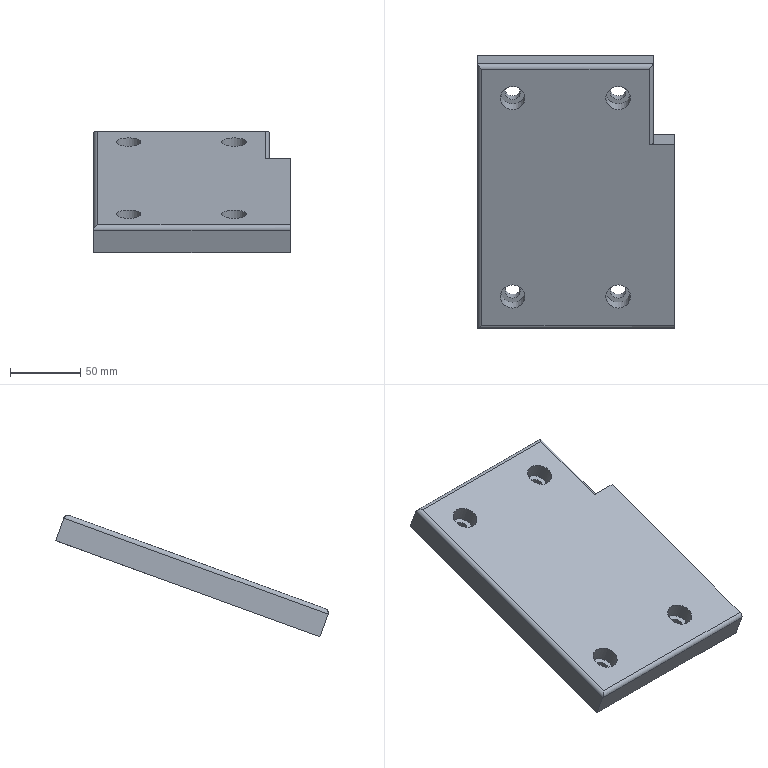Part | NX | features solid 2 | 1 solid | 24 faces | box 140 x 193.934 x 86.353 mm | volume 526407 mm3 | plane 12 | cylinder 12 | commonest cylinder face diameters 6 x4 11 x4 17.5 x4
STEP:
#1=CARTESIAN_POINT('',(540.,942.377,-265.264));
#2=VERTEX_POINT('',#1);
#3=CARTESIAN_POINT('',(540.,998.758,-244.742));
#4=VERTEX_POINT('',#3);
#5=CARTESIAN_POINT('',(540.,810.726,-313.181));
#6=DIRECTION('',(0.,0.9397,0.342));
#7=VECTOR('',#6,1000.);
#8=LINE('',#5,#7);
#9=EDGE_CURVE('',#2,#4,#8,.T.);
#10=ORIENTED_EDGE('',*,*,#9,.F.);
#11=CARTESIAN_POINT('',(540.,948.191,-281.238));
#12=VERTEX_POINT('',#11);
#13=CARTESIAN_POINT('',(540.,941.316,-262.351));
#14=DIRECTION('',(0.,0.342,-0.9397));
#15=VECTOR('',#14,1000.);
#16=LINE('',#13,#15);
#17=EDGE_CURVE('',#2,#12,#16,.T.);
#18=ORIENTED_EDGE('',*,*,#17,.T.);
#19=CARTESIAN_POINT('',(540.,1004.573,-260.717));
#20=VERTEX_POINT('',#19);
#21=CARTESIAN_POINT('',(540.,816.446,-329.19));
#22=DIRECTION('',(0.,0.9397,0.342));
#23=VECTOR('',#22,1000.);
#24=LINE('',#21,#23);
#25=EDGE_CURVE('',#12,#20,#24,.T.);
#26=ORIENTED_EDGE('',*,*,#25,.T.);
#27=CARTESIAN_POINT('',(540.,997.698,-241.829));
#28=DIRECTION('',(0.,0.342,-0.9397));
#29=VECTOR('',#28,1000.);
#30=LINE('',#27,#29);
#31=EDGE_CURVE('',#4,#20,#30,.T.);
#32=ORIENTED_EDGE('',*,*,#31,.F.);
#33=EDGE_LOOP('',(#10,#18,#26,#32));
#34=FACE_BOUND('',#33,.T.);
#35=CARTESIAN_POINT('',(540.,809.665,-310.268));
#36=DIRECTION('',(1.,0.,0.));
#37=DIRECTION('',(0.,0.9397,0.342));
#38=AXIS2_PLACEMENT_3D('',#35,#36,#37);
#39=PLANE('',#38);
#40=ADVANCED_FACE('',(#34),#39,.T.);
#41=CARTESIAN_POINT('',(415.,810.82,-313.146));
#42=VERTEX_POINT('',#41);
#43=CARTESIAN_POINT('',(555.,810.82,-313.146));
#44=VERTEX_POINT('',#43);
#45=CARTESIAN_POINT('',(543.95,810.82,-313.146));
#46=DIRECTION('',(-1.,0.,0.));
#47=VECTOR('',#46,1000.);
#48=LINE('',#45,#47);
#49=EDGE_CURVE('',#42,#44,#48,.F.);
#50=ORIENTED_EDGE('',*,*,#49,.T.);
#51=CARTESIAN_POINT('',(555.,812.613,-309.301));
#52=VERTEX_POINT('',#51);
#53=CARTESIAN_POINT('',(555.,813.639,-312.12));
#54=DIRECTION('',(1.,0.,0.));
#55=DIRECTION('',(0.,1.,0.));
#56=AXIS2_PLACEMENT_3D('',#53,#54,#55);
#57=CIRCLE('',#56,3.);
#58=EDGE_CURVE('',#44,#52,#57,.F.);
#59=ORIENTED_EDGE('',*,*,#58,.T.);
#60=CARTESIAN_POINT('',(418.,812.613,-309.301));
#61=VERTEX_POINT('',#60);
#62=CARTESIAN_POINT('',(427.4,812.613,-309.301));
#63=DIRECTION('',(-1.,0.,0.));
#64=VECTOR('',#63,1000.);
#65=LINE('',#62,#64);
#66=EDGE_CURVE('',#52,#61,#65,.T.);
#67=ORIENTED_EDGE('',*,*,#66,.T.);
#68=CARTESIAN_POINT('',(418.,813.639,-312.12));
#69=DIRECTION('',(0.7071,-0.6645,-0.2418));
#70=DIRECTION('',(-0.7071,-0.6645,-0.2418));
#71=AXIS2_PLACEMENT_3D('',#68,#69,#70);
#72=ELLIPSE('',#71,4.243,3.);
#73=EDGE_CURVE('',#61,#42,#72,.T.);
#74=ORIENTED_EDGE('',*,*,#73,.T.);
#75=EDGE_LOOP('',(#50,#59,#67,#74));
#76=FACE_BOUND('',#75,.T.);
#77=CARTESIAN_POINT('',(427.4,813.639,-312.12));
#78=DIRECTION('',(-1.,0.,0.));
#79=DIRECTION('',(0.,1.,0.));
#80=AXIS2_PLACEMENT_3D('',#77,#78,#79);
#81=CYLINDRICAL_SURFACE('',#80,3.);
#82=ADVANCED_FACE('',(#76),#81,.T.);
#83=CARTESIAN_POINT('',(537.,994.913,-242.949));
#84=VERTEX_POINT('',#83);
#85=CARTESIAN_POINT('',(537.,941.351,-262.444));
#86=VERTEX_POINT('',#85);
#87=CARTESIAN_POINT('',(537.,809.606,-310.396));
#88=DIRECTION('',(0.,0.9397,0.342));
#89=VECTOR('',#88,1000.);
#90=LINE('',#87,#89);
#91=EDGE_CURVE('',#84,#86,#90,.F.);
#92=ORIENTED_EDGE('',*,*,#91,.T.);
#93=CARTESIAN_POINT('',(537.,942.377,-265.264));
#94=DIRECTION('',(0.,-0.9397,-0.342));
#95=DIRECTION('',(-0.0602,0.3414,-0.938));
#96=AXIS2_PLACEMENT_3D('',#93,#94,#95);
#97=CIRCLE('',#96,3.);
#98=EDGE_CURVE('',#86,#2,#97,.F.);
#99=ORIENTED_EDGE('',*,*,#98,.T.);
#100=ORIENTED_EDGE('',*,*,#9,.T.);
#101=CARTESIAN_POINT('',(537.,995.939,-245.768));
#102=DIRECTION('',(0.7071,-0.6645,-0.2418));
#103=DIRECTION('',(0.7071,0.6645,0.2418));
#104=AXIS2_PLACEMENT_3D('',#101,#102,#103);
#105=ELLIPSE('',#104,4.243,3.);
#106=EDGE_CURVE('',#4,#84,#105,.T.);
#107=ORIENTED_EDGE('',*,*,#106,.T.);
#108=EDGE_LOOP('',(#92,#99,#100,#107));
#109=FACE_BOUND('',#108,.T.);
#110=CARTESIAN_POINT('',(537.,810.726,-313.181));
#111=DIRECTION('',(0.,0.9397,0.342));
#112=DIRECTION('',(0.,-0.342,0.9397));
#113=AXIS2_PLACEMENT_3D('',#110,#111,#112);
#114=CYLINDRICAL_SURFACE('',#113,3.);
#115=ADVANCED_FACE('',(#109),#114,.T.);
#116=CARTESIAN_POINT('',(555.,941.351,-262.444));
#117=VERTEX_POINT('',#116);
#118=CARTESIAN_POINT('',(540.,941.351,-262.444));
#119=DIRECTION('',(-1.,0.,0.));
#120=VECTOR('',#119,1000.);
#121=LINE('',#118,#120);
#122=EDGE_CURVE('',#86,#117,#121,.F.);
#123=ORIENTED_EDGE('',*,*,#122,.F.);
#124=ORIENTED_EDGE('',*,*,#91,.F.);
#125=CARTESIAN_POINT('',(418.,994.913,-242.949));
#126=VERTEX_POINT('',#125);
#127=CARTESIAN_POINT('',(427.4,994.913,-242.949));
#128=DIRECTION('',(-1.,0.,0.));
#129=VECTOR('',#128,1000.);
#130=LINE('',#127,#129);
#131=EDGE_CURVE('',#126,#84,#130,.F.);
#132=ORIENTED_EDGE('',*,*,#131,.F.);
#133=CARTESIAN_POINT('',(418.,809.606,-310.396));
#134=DIRECTION('',(0.,0.9397,0.342));
#135=VECTOR('',#134,1000.);
#136=LINE('',#133,#135);
#137=EDGE_CURVE('',#61,#126,#136,.T.);
#138=ORIENTED_EDGE('',*,*,#137,.F.);
#139=ORIENTED_EDGE('',*,*,#66,.F.);
#140=CARTESIAN_POINT('',(555.,809.7,-310.362));
#141=DIRECTION('',(0.,-0.9397,-0.342));
#142=VECTOR('',#141,1000.);
#143=LINE('',#140,#142);
#144=EDGE_CURVE('',#52,#117,#143,.F.);
#145=ORIENTED_EDGE('',*,*,#144,.T.);
#146=EDGE_LOOP('',(#123,#124,#132,#138,#139,#145));
#147=FACE_BOUND('',#146,.T.);
#148=CARTESIAN_POINT('',(440.,841.508,-298.784));
#149=VERTEX_POINT('',#148);
#150=CARTESIAN_POINT('',(440.,833.286,-301.777));
#151=DIRECTION('',(0.,-0.342,0.9397));
#152=DIRECTION('',(0.,0.9397,0.342));
#153=AXIS2_PLACEMENT_3D('',#150,#151,#152);
#154=CIRCLE('',#153,8.75);
#155=EDGE_CURVE('',#149,#149,#154,.T.);
#156=ORIENTED_EDGE('',*,*,#155,.F.);
#157=EDGE_LOOP('',(#156));
#158=FACE_BOUND('',#157,.T.);
#159=CARTESIAN_POINT('',(515.,841.508,-298.784));
#160=VERTEX_POINT('',#159);
#161=CARTESIAN_POINT('',(515.,833.286,-301.777));
#162=DIRECTION('',(0.,-0.342,0.9397));
#163=DIRECTION('',(0.,0.9397,0.342));
#164=AXIS2_PLACEMENT_3D('',#161,#162,#163);
#165=CIRCLE('',#164,8.75);
#166=EDGE_CURVE('',#160,#160,#165,.T.);
#167=ORIENTED_EDGE('',*,*,#166,.F.);
#168=EDGE_LOOP('',(#167));
#169=FACE_BOUND('',#168,.T.);
#170=CARTESIAN_POINT('',(515.,966.018,-253.466));
#171=VERTEX_POINT('',#170);
#172=CARTESIAN_POINT('',(515.,974.24,-250.474));
#173=DIRECTION('',(0.,0.342,-0.9397));
#174=DIRECTION('',(0.,-0.9397,-0.342));
#175=AXIS2_PLACEMENT_3D('',#172,#173,#174);
#176=CIRCLE('',#175,8.75);
#177=EDGE_CURVE('',#171,#171,#176,.F.);
#178=ORIENTED_EDGE('',*,*,#177,.F.);
#179=EDGE_LOOP('',(#178));
#180=FACE_BOUND('',#179,.T.);
#181=CARTESIAN_POINT('',(440.,966.018,-253.466));
#182=VERTEX_POINT('',#181);
#183=CARTESIAN_POINT('',(440.,974.24,-250.474));
#184=DIRECTION('',(0.,0.342,-0.9397));
#185=DIRECTION('',(0.,-0.9397,-0.342));
#186=AXIS2_PLACEMENT_3D('',#183,#184,#185);
#187=CIRCLE('',#186,8.75);
#188=EDGE_CURVE('',#182,#182,#187,.F.);
#189=ORIENTED_EDGE('',*,*,#188,.F.);
#190=EDGE_LOOP('',(#189));
#191=FACE_BOUND('',#190,.T.);
#192=CARTESIAN_POINT('',(427.4,809.606,-310.396));
#193=DIRECTION('',(0.,-0.342,0.9397));
#194=DIRECTION('',(0.,0.9397,0.342));
#195=AXIS2_PLACEMENT_3D('',#192,#193,#194);
#196=PLANE('',#195);
#197=ADVANCED_FACE('',(#147,#158,#169,#180,#191),#196,.T.);
#198=CARTESIAN_POINT('',(555.,816.634,-329.121));
#199=VERTEX_POINT('',#198);
#200=CARTESIAN_POINT('',(555.,809.759,-310.233));
#201=DIRECTION('',(0.,-0.342,0.9397));
#202=VECTOR('',#201,1000.);
#203=LINE('',#200,#202);
#204=EDGE_CURVE('',#199,#44,#203,.T.);
#205=ORIENTED_EDGE('',*,*,#204,.T.);
#206=ORIENTED_EDGE('',*,*,#49,.F.);
#207=CARTESIAN_POINT('',(415.,816.634,-329.121));
#208=VERTEX_POINT('',#207);
#209=CARTESIAN_POINT('',(415.,817.01,-330.155));
#210=DIRECTION('',(0.,-0.342,0.9397));
#211=VECTOR('',#210,1000.);
#212=LINE('',#209,#211);
#213=EDGE_CURVE('',#208,#42,#212,.T.);
#214=ORIENTED_EDGE('',*,*,#213,.F.);
#215=CARTESIAN_POINT('',(427.5,816.634,-329.121));
#216=DIRECTION('',(1.,0.,0.));
#217=VECTOR('',#216,1000.);
#218=LINE('',#215,#217);
#219=EDGE_CURVE('',#208,#199,#218,.T.);
#220=ORIENTED_EDGE('',*,*,#219,.T.);
#221=EDGE_LOOP('',(#205,#206,#214,#220));
#222=FACE_BOUND('',#221,.T.);
#223=CARTESIAN_POINT('',(543.95,817.01,-330.155));
#224=DIRECTION('',(0.,-0.9397,-0.342));
#225=DIRECTION('',(-1.,0.,0.));
#226=AXIS2_PLACEMENT_3D('',#223,#224,#225);
#227=PLANE('',#226);
#228=ADVANCED_FACE('',(#222),#227,.T.);
#229=ORIENTED_EDGE('',*,*,#25,.F.);
#230=CARTESIAN_POINT('',(555.,948.191,-281.238));
#231=VERTEX_POINT('',#230);
#232=CARTESIAN_POINT('',(540.,948.191,-281.238));
#233=DIRECTION('',(1.,0.,0.));
#234=VECTOR('',#233,1000.);
#235=LINE('',#232,#234);
#236=EDGE_CURVE('',#12,#231,#235,.T.);
#237=ORIENTED_EDGE('',*,*,#236,.T.);
#238=CARTESIAN_POINT('',(555.,816.446,-329.19));
#239=DIRECTION('',(0.,0.9397,0.342));
#240=VECTOR('',#239,1000.);
#241=LINE('',#238,#240);
#242=EDGE_CURVE('',#199,#231,#241,.T.);
#243=ORIENTED_EDGE('',*,*,#242,.F.);
#244=ORIENTED_EDGE('',*,*,#219,.F.);
#245=CARTESIAN_POINT('',(415.,1004.573,-260.717));
#246=VERTEX_POINT('',#245);
#247=CARTESIAN_POINT('',(415.,816.446,-329.19));
#248=DIRECTION('',(0.,-0.9397,-0.342));
#249=VECTOR('',#248,1000.);
#250=LINE('',#247,#249);
#251=EDGE_CURVE('',#246,#208,#250,.T.);
#252=ORIENTED_EDGE('',*,*,#251,.F.);
#253=CARTESIAN_POINT('',(526.6,1004.573,-260.717));
#254=DIRECTION('',(1.,0.,0.));
#255=VECTOR('',#254,1000.);
#256=LINE('',#253,#255);
#257=EDGE_CURVE('',#246,#20,#256,.T.);
#258=ORIENTED_EDGE('',*,*,#257,.T.);
#259=EDGE_LOOP('',(#229,#237,#243,#244,#252,#258));
#260=FACE_BOUND('',#259,.T.);
#261=CARTESIAN_POINT('',(440.,845.295,-318.69));
#262=VERTEX_POINT('',#261);
#263=CARTESIAN_POINT('',(440.,840.126,-320.571));
#264=DIRECTION('',(0.,-0.342,0.9397));
#265=DIRECTION('',(0.,0.9397,0.342));
#266=AXIS2_PLACEMENT_3D('',#263,#264,#265);
#267=CIRCLE('',#266,5.5);
#268=EDGE_CURVE('',#262,#262,#267,.T.);
#269=ORIENTED_EDGE('',*,*,#268,.T.);
#270=EDGE_LOOP('',(#269));
#271=FACE_BOUND('',#270,.T.);
#272=CARTESIAN_POINT('',(515.,845.295,-318.69));
#273=VERTEX_POINT('',#272);
#274=CARTESIAN_POINT('',(515.,840.126,-320.571));
#275=DIRECTION('',(0.,-0.342,0.9397));
#276=DIRECTION('',(0.,0.9397,0.342));
#277=AXIS2_PLACEMENT_3D('',#274,#275,#276);
#278=CIRCLE('',#277,5.5);
#279=EDGE_CURVE('',#273,#273,#278,.T.);
#280=ORIENTED_EDGE('',*,*,#279,.T.);
#281=EDGE_LOOP('',(#280));
#282=FACE_BOUND('',#281,.T.);
#283=CARTESIAN_POINT('',(515.,986.249,-267.387));
#284=VERTEX_POINT('',#283);
#285=CARTESIAN_POINT('',(515.,981.08,-269.268));
#286=DIRECTION('',(0.,-0.342,0.9397));
#287=DIRECTION('',(0.,0.9397,0.342));
#288=AXIS2_PLACEMENT_3D('',#285,#286,#287);
#289=CIRCLE('',#288,5.5);
#290=EDGE_CURVE('',#284,#284,#289,.T.);
#291=ORIENTED_EDGE('',*,*,#290,.T.);
#292=EDGE_LOOP('',(#291));
#293=FACE_BOUND('',#292,.T.);
#294=CARTESIAN_POINT('',(440.,986.249,-267.387));
#295=VERTEX_POINT('',#294);
#296=CARTESIAN_POINT('',(440.,981.08,-269.268));
#297=DIRECTION('',(0.,-0.342,0.9397));
#298=DIRECTION('',(0.,0.9397,0.342));
#299=AXIS2_PLACEMENT_3D('',#296,#297,#298);
#300=CIRCLE('',#299,5.5);
#301=EDGE_CURVE('',#295,#295,#300,.T.);
#302=ORIENTED_EDGE('',*,*,#301,.T.);
#303=EDGE_LOOP('',(#302));
#304=FACE_BOUND('',#303,.T.);
#305=CARTESIAN_POINT('',(544.05,816.446,-329.19));
#306=DIRECTION('',(0.,0.342,-0.9397));
#307=DIRECTION('',(0.,0.9397,0.342));
#308=AXIS2_PLACEMENT_3D('',#305,#306,#307);
#309=PLANE('',#308);
#310=ADVANCED_FACE('',(#260,#271,#282,#293,#304),#309,.T.);
#311=ORIENTED_EDGE('',*,*,#31,.T.);
#312=ORIENTED_EDGE('',*,*,#257,.F.);
#313=CARTESIAN_POINT('',(415.,998.758,-244.742));
#314=VERTEX_POINT('',#313);
#315=CARTESIAN_POINT('',(415.,997.698,-241.829));
#316=DIRECTION('',(0.,0.342,-0.9397));
#317=VECTOR('',#316,1000.);
#318=LINE('',#315,#317);
#319=EDGE_CURVE('',#314,#246,#318,.T.);
#320=ORIENTED_EDGE('',*,*,#319,.F.);
#321=CARTESIAN_POINT('',(526.6,998.758,-244.742));
#322=DIRECTION('',(-1.,0.,0.));
#323=VECTOR('',#322,1000.);
#324=LINE('',#321,#323);
#325=EDGE_CURVE('',#4,#314,#324,.T.);
#326=ORIENTED_EDGE('',*,*,#325,.F.);
#327=EDGE_LOOP('',(#311,#312,#320,#326));
#328=FACE_BOUND('',#327,.T.);
#329=CARTESIAN_POINT('',(526.6,997.698,-241.829));
#330=DIRECTION('',(0.,0.9397,0.342));
#331=DIRECTION('',(-1.,0.,0.));
#332=AXIS2_PLACEMENT_3D('',#329,#330,#331);
#333=PLANE('',#332);
#334=ADVANCED_FACE('',(#328),#333,.T.);
#335=ORIENTED_EDGE('',*,*,#319,.T.);
#336=ORIENTED_EDGE('',*,*,#251,.T.);
#337=ORIENTED_EDGE('',*,*,#213,.T.);
#338=CARTESIAN_POINT('',(415.,803.772,-315.712));
#339=DIRECTION('',(0.,0.9397,0.342));
#340=VECTOR('',#339,1000.);
#341=LINE('',#338,#340);
#342=EDGE_CURVE('',#314,#42,#341,.F.);
#343=ORIENTED_EDGE('',*,*,#342,.F.);
#344=EDGE_LOOP('',(#335,#336,#337,#343));
#345=FACE_BOUND('',#344,.T.);
#346=CARTESIAN_POINT('',(415.,809.928,-332.626));
#347=DIRECTION('',(-1.,0.,0.));
#348=DIRECTION('',(0.,0.9397,0.342));
#349=AXIS2_PLACEMENT_3D('',#346,#347,#348);
#350=PLANE('',#349);
#351=ADVANCED_FACE('',(#345),#350,.T.);
#352=ORIENTED_EDGE('',*,*,#268,.F.);
#353=EDGE_LOOP('',(#352));
#354=FACE_BOUND('',#353,.T.);
#355=CARTESIAN_POINT('',(440.,842.558,-311.172));
#356=VERTEX_POINT('',#355);
#357=CARTESIAN_POINT('',(440.,837.39,-313.053));
#358=DIRECTION('',(0.,-0.342,0.9397));
#359=DIRECTION('',(0.,0.9397,0.342));
#360=AXIS2_PLACEMENT_3D('',#357,#358,#359);
#361=CIRCLE('',#360,5.5);
#362=EDGE_CURVE('',#356,#356,#361,.T.);
#363=ORIENTED_EDGE('',*,*,#362,.T.);
#364=EDGE_LOOP('',(#363));
#365=FACE_BOUND('',#364,.T.);
#366=CARTESIAN_POINT('',(440.,850.387,-348.761));
#367=DIRECTION('',(0.,0.342,-0.9397));
#368=DIRECTION('',(0.,0.9397,0.342));
#369=AXIS2_PLACEMENT_3D('',#366,#367,#368);
#370=CYLINDRICAL_SURFACE('',#369,5.5);
#371=ADVANCED_FACE('',(#354,#365),#370,.F.);
#372=ORIENTED_EDGE('',*,*,#362,.F.);
#373=EDGE_LOOP('',(#372));
#374=FACE_BOUND('',#373,.T.);
#375=CARTESIAN_POINT('',(440.,845.612,-310.06));
#376=VERTEX_POINT('',#375);
#377=CARTESIAN_POINT('',(440.,837.39,-313.053));
#378=DIRECTION('',(0.,-0.342,0.9397));
#379=DIRECTION('',(0.,0.9397,0.342));
#380=AXIS2_PLACEMENT_3D('',#377,#378,#379);
#381=CIRCLE('',#380,8.75);
#382=EDGE_CURVE('',#376,#376,#381,.T.);
#383=ORIENTED_EDGE('',*,*,#382,.T.);
#384=EDGE_LOOP('',(#383));
#385=FACE_BOUND('',#384,.T.);
#386=CARTESIAN_POINT('',(452.,837.39,-313.053));
#387=DIRECTION('',(0.,0.342,-0.9397));
#388=DIRECTION('',(0.,0.9397,0.342));
#389=AXIS2_PLACEMENT_3D('',#386,#387,#388);
#390=PLANE('',#389);
#391=ADVANCED_FACE('',(#374,#385),#390,.F.);
#392=ORIENTED_EDGE('',*,*,#382,.F.);
#393=EDGE_LOOP('',(#392));
#394=FACE_BOUND('',#393,.T.);
#395=ORIENTED_EDGE('',*,*,#155,.T.);
#396=EDGE_LOOP('',(#395));
#397=FACE_BOUND('',#396,.T.);
#398=CARTESIAN_POINT('',(440.,833.286,-301.777));
#399=DIRECTION('',(0.,0.342,-0.9397));
#400=DIRECTION('',(0.,0.9397,0.342));
#401=AXIS2_PLACEMENT_3D('',#398,#399,#400);
#402=CYLINDRICAL_SURFACE('',#401,8.75);
#403=ADVANCED_FACE('',(#394,#397),#402,.F.);
#404=ORIENTED_EDGE('',*,*,#279,.F.);
#405=EDGE_LOOP('',(#404));
#406=FACE_BOUND('',#405,.T.);
#407=CARTESIAN_POINT('',(515.,842.558,-311.172));
#408=VERTEX_POINT('',#407);
#409=CARTESIAN_POINT('',(515.,837.39,-313.053));
#410=DIRECTION('',(0.,-0.342,0.9397));
#411=DIRECTION('',(0.,0.9397,0.342));
#412=AXIS2_PLACEMENT_3D('',#409,#410,#411);
#413=CIRCLE('',#412,5.5);
#414=EDGE_CURVE('',#408,#408,#413,.T.);
#415=ORIENTED_EDGE('',*,*,#414,.T.);
#416=EDGE_LOOP('',(#415));
#417=FACE_BOUND('',#416,.T.);
#418=CARTESIAN_POINT('',(515.,850.387,-348.761));
#419=DIRECTION('',(0.,0.342,-0.9397));
#420=DIRECTION('',(0.,0.9397,0.342));
#421=AXIS2_PLACEMENT_3D('',#418,#419,#420);
#422=CYLINDRICAL_SURFACE('',#421,5.5);
#423=ADVANCED_FACE('',(#406,#417),#422,.F.);
#424=ORIENTED_EDGE('',*,*,#414,.F.);
#425=EDGE_LOOP('',(#424));
#426=FACE_BOUND('',#425,.T.);
#427=CARTESIAN_POINT('',(515.,845.612,-310.06));
#428=VERTEX_POINT('',#427);
#429=CARTESIAN_POINT('',(515.,837.39,-313.053));
#430=DIRECTION('',(0.,-0.342,0.9397));
#431=DIRECTION('',(0.,0.9397,0.342));
#432=AXIS2_PLACEMENT_3D('',#429,#430,#431);
#433=CIRCLE('',#432,8.75);
#434=EDGE_CURVE('',#428,#428,#433,.T.);
#435=ORIENTED_EDGE('',*,*,#434,.T.);
#436=EDGE_LOOP('',(#435));
#437=FACE_BOUND('',#436,.T.);
#438=CARTESIAN_POINT('',(502.,837.39,-313.053));
#439=DIRECTION('',(0.,0.342,-0.9397));
#440=DIRECTION('',(0.,0.9397,0.342));
#441=AXIS2_PLACEMENT_3D('',#438,#439,#440);
#442=PLANE('',#441);
#443=ADVANCED_FACE('',(#426,#437),#442,.F.);
#444=ORIENTED_EDGE('',*,*,#434,.F.);
#445=EDGE_LOOP('',(#444));
#446=FACE_BOUND('',#445,.T.);
#447=ORIENTED_EDGE('',*,*,#166,.T.);
#448=EDGE_LOOP('',(#447));
#449=FACE_BOUND('',#448,.T.);
#450=CARTESIAN_POINT('',(515.,833.286,-301.777));
#451=DIRECTION('',(0.,0.342,-0.9397));
#452=DIRECTION('',(0.,0.9397,0.342));
#453=AXIS2_PLACEMENT_3D('',#450,#451,#452);
#454=CYLINDRICAL_SURFACE('',#453,8.75);
#455=ADVANCED_FACE('',(#446,#449),#454,.F.);
#456=ORIENTED_EDGE('',*,*,#290,.F.);
#457=EDGE_LOOP('',(#456));
#458=FACE_BOUND('',#457,.T.);
#459=CARTESIAN_POINT('',(515.,983.512,-259.869));
#460=VERTEX_POINT('',#459);
#461=CARTESIAN_POINT('',(515.,978.344,-261.75));
#462=DIRECTION('',(0.,-0.342,0.9397));
#463=DIRECTION('',(0.,0.9397,0.342));
#464=AXIS2_PLACEMENT_3D('',#461,#462,#463);
#465=CIRCLE('',#464,5.5);
#466=EDGE_CURVE('',#460,#460,#465,.T.);
#467=ORIENTED_EDGE('',*,*,#466,.T.);
#468=EDGE_LOOP('',(#467));
#469=FACE_BOUND('',#468,.T.);
#470=CARTESIAN_POINT('',(515.,991.341,-297.458));
#471=DIRECTION('',(0.,0.342,-0.9397));
#472=DIRECTION('',(0.,0.9397,0.342));
#473=AXIS2_PLACEMENT_3D('',#470,#471,#472);
#474=CYLINDRICAL_SURFACE('',#473,5.5);
#475=ADVANCED_FACE('',(#458,#469),#474,.F.);
#476=ORIENTED_EDGE('',*,*,#466,.F.);
#477=EDGE_LOOP('',(#476));
#478=FACE_BOUND('',#477,.T.);
#479=CARTESIAN_POINT('',(515.,986.566,-258.757));
#480=VERTEX_POINT('',#479);
#481=CARTESIAN_POINT('',(515.,978.344,-261.75));
#482=DIRECTION('',(0.,-0.342,0.9397));
#483=DIRECTION('',(0.,0.9397,0.342));
#484=AXIS2_PLACEMENT_3D('',#481,#482,#483);
#485=CIRCLE('',#484,8.75);
#486=EDGE_CURVE('',#480,#480,#485,.T.);
#487=ORIENTED_EDGE('',*,*,#486,.T.);
#488=EDGE_LOOP('',(#487));
#489=FACE_BOUND('',#488,.T.);
#490=CARTESIAN_POINT('',(502.,1025.329,-244.649));
#491=DIRECTION('',(0.,0.342,-0.9397));
#492=DIRECTION('',(0.,0.9397,0.342));
#493=AXIS2_PLACEMENT_3D('',#490,#491,#492);
#494=PLANE('',#493);
#495=ADVANCED_FACE('',(#478,#489),#494,.F.);
#496=ORIENTED_EDGE('',*,*,#486,.F.);
#497=EDGE_LOOP('',(#496));
#498=FACE_BOUND('',#497,.T.);
#499=ORIENTED_EDGE('',*,*,#177,.T.);
#500=EDGE_LOOP('',(#499));
#501=FACE_BOUND('',#500,.T.);
#502=CARTESIAN_POINT('',(515.,974.24,-250.474));
#503=DIRECTION('',(0.,0.342,-0.9397));
#504=DIRECTION('',(0.,0.9397,0.342));
#505=AXIS2_PLACEMENT_3D('',#502,#503,#504);
#506=CYLINDRICAL_SURFACE('',#505,8.75);
#507=ADVANCED_FACE('',(#498,#501),#506,.F.);
#508=ORIENTED_EDGE('',*,*,#301,.F.);
#509=EDGE_LOOP('',(#508));
#510=FACE_BOUND('',#509,.T.);
#511=CARTESIAN_POINT('',(440.,983.512,-259.869));
#512=VERTEX_POINT('',#511);
#513=CARTESIAN_POINT('',(440.,978.344,-261.75));
#514=DIRECTION('',(0.,-0.342,0.9397));
#515=DIRECTION('',(0.,0.9397,0.342));
#516=AXIS2_PLACEMENT_3D('',#513,#514,#515);
#517=CIRCLE('',#516,5.5);
#518=EDGE_CURVE('',#512,#512,#517,.T.);
#519=ORIENTED_EDGE('',*,*,#518,.T.);
#520=EDGE_LOOP('',(#519));
#521=FACE_BOUND('',#520,.T.);
#522=CARTESIAN_POINT('',(440.,991.341,-297.458));
#523=DIRECTION('',(0.,0.342,-0.9397));
#524=DIRECTION('',(0.,0.9397,0.342));
#525=AXIS2_PLACEMENT_3D('',#522,#523,#524);
#526=CYLINDRICAL_SURFACE('',#525,5.5);
#527=ADVANCED_FACE('',(#510,#521),#526,.F.);
#528=ORIENTED_EDGE('',*,*,#518,.F.);
#529=EDGE_LOOP('',(#528));
#530=FACE_BOUND('',#529,.T.);
#531=CARTESIAN_POINT('',(440.,986.566,-258.757));
#532=VERTEX_POINT('',#531);
#533=CARTESIAN_POINT('',(440.,978.344,-261.75));
#534=DIRECTION('',(0.,-0.342,0.9397));
#535=DIRECTION('',(0.,0.9397,0.342));
#536=AXIS2_PLACEMENT_3D('',#533,#534,#535);
#537=CIRCLE('',#536,8.75);
#538=EDGE_CURVE('',#532,#532,#537,.T.);
#539=ORIENTED_EDGE('',*,*,#538,.T.);
#540=EDGE_LOOP('',(#539));
#541=FACE_BOUND('',#540,.T.);
#542=CARTESIAN_POINT('',(452.,978.344,-261.75));
#543=DIRECTION('',(0.,0.342,-0.9397));
#544=DIRECTION('',(0.,0.9397,0.342));
#545=AXIS2_PLACEMENT_3D('',#542,#543,#544);
#546=PLANE('',#545);
#547=ADVANCED_FACE('',(#530,#541),#546,.F.);
#548=ORIENTED_EDGE('',*,*,#538,.F.);
#549=EDGE_LOOP('',(#548));
#550=FACE_BOUND('',#549,.T.);
#551=ORIENTED_EDGE('',*,*,#188,.T.);
#552=EDGE_LOOP('',(#551));
#553=FACE_BOUND('',#552,.T.);
#554=CARTESIAN_POINT('',(440.,974.24,-250.474));
#555=DIRECTION('',(0.,0.342,-0.9397));
#556=DIRECTION('',(0.,0.9397,0.342));
#557=AXIS2_PLACEMENT_3D('',#554,#555,#556);
#558=CYLINDRICAL_SURFACE('',#557,8.75);
#559=ADVANCED_FACE('',(#550,#553),#558,.F.);
#560=ORIENTED_EDGE('',*,*,#73,.F.);
#561=ORIENTED_EDGE('',*,*,#137,.T.);
#562=CARTESIAN_POINT('',(418.,995.939,-245.768));
#563=DIRECTION('',(-0.7071,-0.6645,-0.2418));
#564=DIRECTION('',(-0.7071,0.6645,0.2418));
#565=AXIS2_PLACEMENT_3D('',#562,#563,#564);
#566=ELLIPSE('',#565,4.243,3.);
#567=EDGE_CURVE('',#126,#314,#566,.T.);
#568=ORIENTED_EDGE('',*,*,#567,.T.);
#569=ORIENTED_EDGE('',*,*,#342,.T.);
#570=EDGE_LOOP('',(#560,#561,#568,#569));
#571=FACE_BOUND('',#570,.T.);
#572=CARTESIAN_POINT('',(418.,810.632,-313.215));
#573=DIRECTION('',(0.,0.9397,0.342));
#574=DIRECTION('',(0.,-0.342,0.9397));
#575=AXIS2_PLACEMENT_3D('',#572,#573,#574);
#576=CYLINDRICAL_SURFACE('',#575,3.);
#577=ADVANCED_FACE('',(#571),#576,.T.);
#578=ORIENTED_EDGE('',*,*,#106,.F.);
#579=ORIENTED_EDGE('',*,*,#325,.T.);
#580=ORIENTED_EDGE('',*,*,#567,.F.);
#581=ORIENTED_EDGE('',*,*,#131,.T.);
#582=EDGE_LOOP('',(#578,#579,#580,#581));
#583=FACE_BOUND('',#582,.T.);
#584=CARTESIAN_POINT('',(526.6,995.939,-245.768));
#585=DIRECTION('',(-1.,0.,0.));
#586=DIRECTION('',(0.,1.,0.));
#587=AXIS2_PLACEMENT_3D('',#584,#585,#586);
#588=CYLINDRICAL_SURFACE('',#587,3.);
#589=ADVANCED_FACE('',(#583),#588,.T.);
#590=ORIENTED_EDGE('',*,*,#17,.F.);
#591=ORIENTED_EDGE('',*,*,#98,.F.);
#592=ORIENTED_EDGE('',*,*,#122,.T.);
#593=CARTESIAN_POINT('',(555.,941.316,-262.351));
#594=DIRECTION('',(0.,0.342,-0.9397));
#595=VECTOR('',#594,1000.);
#596=LINE('',#593,#595);
#597=EDGE_CURVE('',#117,#231,#596,.T.);
#598=ORIENTED_EDGE('',*,*,#597,.T.);
#599=ORIENTED_EDGE('',*,*,#236,.F.);
#600=EDGE_LOOP('',(#590,#591,#592,#598,#599));
#601=FACE_BOUND('',#600,.T.);
#602=CARTESIAN_POINT('',(540.,941.316,-262.351));
#603=DIRECTION('',(0.,-0.9397,-0.342));
#604=DIRECTION('',(-0.0602,0.3414,-0.938));
#605=AXIS2_PLACEMENT_3D('',#602,#603,#604);
#606=PLANE('',#605);
#607=ADVANCED_FACE('',(#601),#606,.F.);
#608=ORIENTED_EDGE('',*,*,#58,.F.);
#609=ORIENTED_EDGE('',*,*,#204,.F.);
#610=ORIENTED_EDGE('',*,*,#242,.T.);
#611=ORIENTED_EDGE('',*,*,#597,.F.);
#612=ORIENTED_EDGE('',*,*,#144,.F.);
#613=EDGE_LOOP('',(#608,#609,#610,#611,#612));
#614=FACE_BOUND('',#613,.T.);
#615=CARTESIAN_POINT('',(555.,809.665,-310.268));
#616=DIRECTION('',(1.,0.,0.));
#617=DIRECTION('',(0.,0.9397,0.342));
#618=AXIS2_PLACEMENT_3D('',#615,#616,#617);
#619=PLANE('',#618);
#620=ADVANCED_FACE('',(#614),#619,.T.);
#621=CLOSED_SHELL('',(#40,#82,#115,#197,#228,#310,#334,#351,#371,#391,#403,#423,#443,#455,#475,#495,#507,#527,#547,#559,#577,#589,#607,#620));
#622=MANIFOLD_SOLID_BREP('',#621);
#623=(LENGTH_UNIT()NAMED_UNIT(*)SI_UNIT(.MILLI.,.METRE.));
#624=UNCERTAINTY_MEASURE_WITH_UNIT(LENGTH_MEASURE(0.00001),#623,'','');
#625=(NAMED_UNIT(*)PLANE_ANGLE_UNIT()SI_UNIT($,.RADIAN.));
#626=(NAMED_UNIT(*)SI_UNIT($,.STERADIAN.)SOLID_ANGLE_UNIT());
#627=(GEOMETRIC_REPRESENTATION_CONTEXT(3)GLOBAL_UNCERTAINTY_ASSIGNED_CONTEXT((#624))GLOBAL_UNIT_ASSIGNED_CONTEXT((#623,#625,#626))REPRESENTATION_CONTEXT('',''));
#628=ADVANCED_BREP_SHAPE_REPRESENTATION('',(#622),#627);